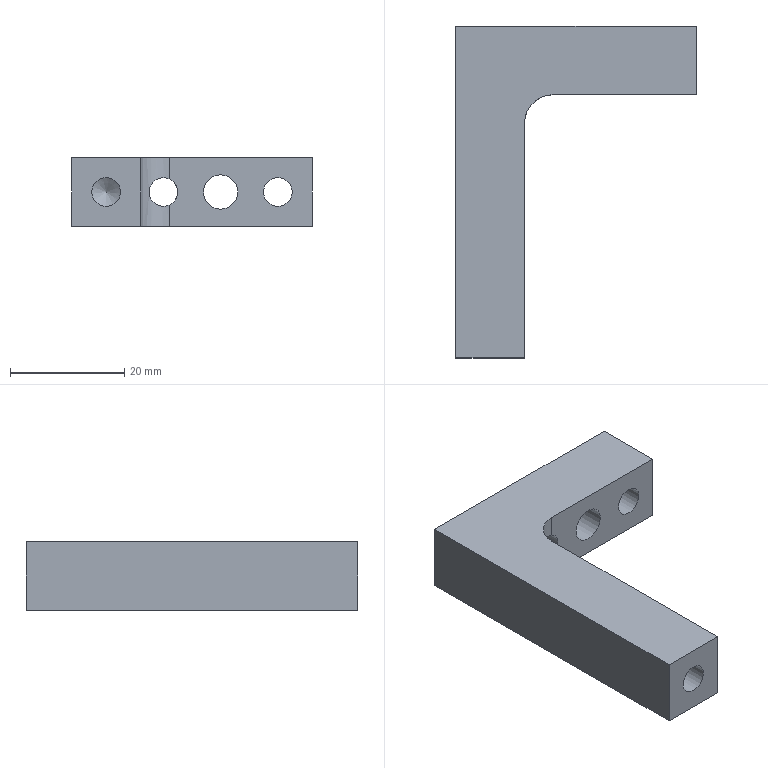Part | NX | features BREP 1 | 1 solid | 16 faces | box 42 x 58 x 12 mm | volume 11260 mm3 | plane 8 | cylinder 6 | cone 2 | commonest cylinder face diameters 5 x3 6 x2 10 x1
STEP:
#1=CARTESIAN_POINT('',(6.,0.,-3.5));
#2=VERTEX_POINT('',#1);
#3=CARTESIAN_POINT('',(6.,0.,-6.));
#4=DIRECTION('',(0.,1.,0.));
#5=DIRECTION('',(0.,0.,1.));
#6=AXIS2_PLACEMENT_3D('',#3,#4,#5);
#7=CIRCLE('',#6,2.5);
#8=EDGE_CURVE('',#2,#2,#7,.T.);
#9=ORIENTED_EDGE('',*,*,#8,.T.);
#10=EDGE_LOOP('',(#9));
#11=FACE_BOUND('',#10,.T.);
#12=CARTESIAN_POINT('',(0.,0.,0.));
#13=VERTEX_POINT('',#12);
#14=CARTESIAN_POINT('',(12.,0.,0.));
#15=VERTEX_POINT('',#14);
#16=CARTESIAN_POINT('',(12.,0.,0.));
#17=DIRECTION('',(1.,0.,0.));
#18=VECTOR('',#17,1000.);
#19=LINE('',#16,#18);
#20=EDGE_CURVE('',#13,#15,#19,.T.);
#21=ORIENTED_EDGE('',*,*,#20,.F.);
#22=CARTESIAN_POINT('',(0.,0.,-12.));
#23=VERTEX_POINT('',#22);
#24=CARTESIAN_POINT('',(0.,0.,-12.));
#25=DIRECTION('',(0.,0.,1.));
#26=VECTOR('',#25,1000.);
#27=LINE('',#24,#26);
#28=EDGE_CURVE('',#23,#13,#27,.T.);
#29=ORIENTED_EDGE('',*,*,#28,.F.);
#30=CARTESIAN_POINT('',(12.,0.,-12.));
#31=VERTEX_POINT('',#30);
#32=CARTESIAN_POINT('',(12.,0.,-12.));
#33=DIRECTION('',(1.,0.,0.));
#34=VECTOR('',#33,1000.);
#35=LINE('',#32,#34);
#36=EDGE_CURVE('',#23,#31,#35,.T.);
#37=ORIENTED_EDGE('',*,*,#36,.T.);
#38=CARTESIAN_POINT('',(12.,0.,-12.));
#39=DIRECTION('',(0.,0.,1.));
#40=VECTOR('',#39,1000.);
#41=LINE('',#38,#40);
#42=EDGE_CURVE('',#31,#15,#41,.T.);
#43=ORIENTED_EDGE('',*,*,#42,.T.);
#44=EDGE_LOOP('',(#21,#29,#37,#43));
#45=FACE_BOUND('',#44,.T.);
#46=CARTESIAN_POINT('',(12.,0.,-12.));
#47=DIRECTION('',(0.,1.,0.));
#48=DIRECTION('',(1.,0.,0.));
#49=AXIS2_PLACEMENT_3D('',#46,#47,#48);
#50=PLANE('',#49);
#51=ADVANCED_FACE('',(#11,#45),#50,.F.);
#52=CARTESIAN_POINT('',(12.,41.,0.));
#53=VERTEX_POINT('',#52);
#54=CARTESIAN_POINT('',(12.,46.,0.));
#55=DIRECTION('',(0.,1.,0.));
#56=VECTOR('',#55,1000.);
#57=LINE('',#54,#56);
#58=EDGE_CURVE('',#15,#53,#57,.T.);
#59=ORIENTED_EDGE('',*,*,#58,.F.);
#60=ORIENTED_EDGE('',*,*,#42,.F.);
#61=CARTESIAN_POINT('',(12.,41.,-12.));
#62=VERTEX_POINT('',#61);
#63=CARTESIAN_POINT('',(12.,46.,-12.));
#64=DIRECTION('',(0.,1.,0.));
#65=VECTOR('',#64,1000.);
#66=LINE('',#63,#65);
#67=EDGE_CURVE('',#31,#62,#66,.T.);
#68=ORIENTED_EDGE('',*,*,#67,.T.);
#69=CARTESIAN_POINT('',(12.,41.,-12.));
#70=DIRECTION('',(0.,0.,-1.));
#71=VECTOR('',#70,1000.);
#72=LINE('',#69,#71);
#73=EDGE_CURVE('',#53,#62,#72,.T.);
#74=ORIENTED_EDGE('',*,*,#73,.F.);
#75=EDGE_LOOP('',(#59,#60,#68,#74));
#76=FACE_BOUND('',#75,.T.);
#77=CARTESIAN_POINT('',(12.,46.,-12.));
#78=DIRECTION('',(-1.,0.,0.));
#79=DIRECTION('',(0.,1.,0.));
#80=AXIS2_PLACEMENT_3D('',#77,#78,#79);
#81=PLANE('',#80);
#82=ADVANCED_FACE('',(#76),#81,.F.);
#83=CARTESIAN_POINT('',(17.,46.,-12.));
#84=VERTEX_POINT('',#83);
#85=CARTESIAN_POINT('',(42.,46.,-12.));
#86=VERTEX_POINT('',#85);
#87=CARTESIAN_POINT('',(42.,46.,-12.));
#88=DIRECTION('',(1.,0.,0.));
#89=VECTOR('',#88,1000.);
#90=LINE('',#87,#89);
#91=EDGE_CURVE('',#84,#86,#90,.T.);
#92=ORIENTED_EDGE('',*,*,#91,.T.);
#93=CARTESIAN_POINT('',(42.,46.,0.));
#94=VERTEX_POINT('',#93);
#95=CARTESIAN_POINT('',(42.,46.,-12.));
#96=DIRECTION('',(0.,0.,1.));
#97=VECTOR('',#96,1000.);
#98=LINE('',#95,#97);
#99=EDGE_CURVE('',#86,#94,#98,.T.);
#100=ORIENTED_EDGE('',*,*,#99,.T.);
#101=CARTESIAN_POINT('',(17.,46.,0.));
#102=VERTEX_POINT('',#101);
#103=CARTESIAN_POINT('',(42.,46.,0.));
#104=DIRECTION('',(1.,0.,0.));
#105=VECTOR('',#104,1000.);
#106=LINE('',#103,#105);
#107=EDGE_CURVE('',#102,#94,#106,.T.);
#108=ORIENTED_EDGE('',*,*,#107,.F.);
#109=CARTESIAN_POINT('',(17.,46.,-3.709));
#110=VERTEX_POINT('',#109);
#111=CARTESIAN_POINT('',(17.,46.,0.));
#112=DIRECTION('',(0.,0.,1.));
#113=VECTOR('',#112,1000.);
#114=LINE('',#111,#113);
#115=EDGE_CURVE('',#110,#102,#114,.T.);
#116=ORIENTED_EDGE('',*,*,#115,.F.);
#117=CARTESIAN_POINT('',(17.,46.,-8.291));
#118=VERTEX_POINT('',#117);
#119=CARTESIAN_POINT('',(16.,46.,-6.));
#120=DIRECTION('',(0.,-1.,0.));
#121=DIRECTION('',(0.,0.,-1.));
#122=AXIS2_PLACEMENT_3D('',#119,#120,#121);
#123=CIRCLE('',#122,2.5);
#124=EDGE_CURVE('',#118,#110,#123,.T.);
#125=ORIENTED_EDGE('',*,*,#124,.F.);
#126=CARTESIAN_POINT('',(17.,46.,0.));
#127=DIRECTION('',(0.,0.,1.));
#128=VECTOR('',#127,1000.);
#129=LINE('',#126,#128);
#130=EDGE_CURVE('',#84,#118,#129,.T.);
#131=ORIENTED_EDGE('',*,*,#130,.F.);
#132=EDGE_LOOP('',(#92,#100,#108,#116,#125,#131));
#133=FACE_BOUND('',#132,.T.);
#134=CARTESIAN_POINT('',(36.,46.,-8.5));
#135=VERTEX_POINT('',#134);
#136=CARTESIAN_POINT('',(36.,46.,-6.));
#137=DIRECTION('',(0.,-1.,0.));
#138=DIRECTION('',(0.,0.,-1.));
#139=AXIS2_PLACEMENT_3D('',#136,#137,#138);
#140=CIRCLE('',#139,2.5);
#141=EDGE_CURVE('',#135,#135,#140,.T.);
#142=ORIENTED_EDGE('',*,*,#141,.F.);
#143=EDGE_LOOP('',(#142));
#144=FACE_BOUND('',#143,.T.);
#145=CARTESIAN_POINT('',(26.,46.,-9.));
#146=VERTEX_POINT('',#145);
#147=CARTESIAN_POINT('',(26.,46.,-6.));
#148=DIRECTION('',(0.,-1.,0.));
#149=DIRECTION('',(0.,0.,-1.));
#150=AXIS2_PLACEMENT_3D('',#147,#148,#149);
#151=CIRCLE('',#150,3.);
#152=EDGE_CURVE('',#146,#146,#151,.T.);
#153=ORIENTED_EDGE('',*,*,#152,.F.);
#154=EDGE_LOOP('',(#153));
#155=FACE_BOUND('',#154,.T.);
#156=CARTESIAN_POINT('',(42.,46.,-12.));
#157=DIRECTION('',(0.,1.,0.));
#158=DIRECTION('',(0.,0.,1.));
#159=AXIS2_PLACEMENT_3D('',#156,#157,#158);
#160=PLANE('',#159);
#161=ADVANCED_FACE('',(#133,#144,#155),#160,.F.);
#162=CARTESIAN_POINT('',(42.,58.,0.));
#163=VERTEX_POINT('',#162);
#164=CARTESIAN_POINT('',(42.,58.,0.));
#165=DIRECTION('',(0.,1.,0.));
#166=VECTOR('',#165,1000.);
#167=LINE('',#164,#166);
#168=EDGE_CURVE('',#94,#163,#167,.T.);
#169=ORIENTED_EDGE('',*,*,#168,.F.);
#170=ORIENTED_EDGE('',*,*,#99,.F.);
#171=CARTESIAN_POINT('',(42.,58.,-12.));
#172=VERTEX_POINT('',#171);
#173=CARTESIAN_POINT('',(42.,58.,-12.));
#174=DIRECTION('',(0.,1.,0.));
#175=VECTOR('',#174,1000.);
#176=LINE('',#173,#175);
#177=EDGE_CURVE('',#86,#172,#176,.T.);
#178=ORIENTED_EDGE('',*,*,#177,.T.);
#179=CARTESIAN_POINT('',(42.,58.,-12.));
#180=DIRECTION('',(0.,0.,1.));
#181=VECTOR('',#180,1000.);
#182=LINE('',#179,#181);
#183=EDGE_CURVE('',#172,#163,#182,.T.);
#184=ORIENTED_EDGE('',*,*,#183,.T.);
#185=EDGE_LOOP('',(#169,#170,#178,#184));
#186=FACE_BOUND('',#185,.T.);
#187=CARTESIAN_POINT('',(42.,58.,-12.));
#188=DIRECTION('',(-1.,0.,0.));
#189=DIRECTION('',(0.,1.,0.));
#190=AXIS2_PLACEMENT_3D('',#187,#188,#189);
#191=PLANE('',#190);
#192=ADVANCED_FACE('',(#186),#191,.F.);
#193=CARTESIAN_POINT('',(16.,58.,-8.5));
#194=VERTEX_POINT('',#193);
#195=CARTESIAN_POINT('',(16.,58.,-6.));
#196=DIRECTION('',(0.,-1.,0.));
#197=DIRECTION('',(0.,0.,-1.));
#198=AXIS2_PLACEMENT_3D('',#195,#196,#197);
#199=CIRCLE('',#198,2.5);
#200=EDGE_CURVE('',#194,#194,#199,.T.);
#201=ORIENTED_EDGE('',*,*,#200,.T.);
#202=EDGE_LOOP('',(#201));
#203=FACE_BOUND('',#202,.T.);
#204=CARTESIAN_POINT('',(36.,58.,-8.5));
#205=VERTEX_POINT('',#204);
#206=CARTESIAN_POINT('',(36.,58.,-6.));
#207=DIRECTION('',(0.,-1.,0.));
#208=DIRECTION('',(0.,0.,-1.));
#209=AXIS2_PLACEMENT_3D('',#206,#207,#208);
#210=CIRCLE('',#209,2.5);
#211=EDGE_CURVE('',#205,#205,#210,.T.);
#212=ORIENTED_EDGE('',*,*,#211,.T.);
#213=EDGE_LOOP('',(#212));
#214=FACE_BOUND('',#213,.T.);
#215=CARTESIAN_POINT('',(6.,58.,-9.));
#216=VERTEX_POINT('',#215);
#217=CARTESIAN_POINT('',(6.,58.,-6.));
#218=DIRECTION('',(0.,-1.,0.));
#219=DIRECTION('',(0.,0.,-1.));
#220=AXIS2_PLACEMENT_3D('',#217,#218,#219);
#221=CIRCLE('',#220,3.);
#222=EDGE_CURVE('',#216,#216,#221,.T.);
#223=ORIENTED_EDGE('',*,*,#222,.T.);
#224=EDGE_LOOP('',(#223));
#225=FACE_BOUND('',#224,.T.);
#226=CARTESIAN_POINT('',(26.,58.,-9.));
#227=VERTEX_POINT('',#226);
#228=CARTESIAN_POINT('',(26.,58.,-6.));
#229=DIRECTION('',(0.,-1.,0.));
#230=DIRECTION('',(0.,0.,-1.));
#231=AXIS2_PLACEMENT_3D('',#228,#229,#230);
#232=CIRCLE('',#231,3.);
#233=EDGE_CURVE('',#227,#227,#232,.T.);
#234=ORIENTED_EDGE('',*,*,#233,.T.);
#235=EDGE_LOOP('',(#234));
#236=FACE_BOUND('',#235,.T.);
#237=CARTESIAN_POINT('',(0.,58.,0.));
#238=VERTEX_POINT('',#237);
#239=CARTESIAN_POINT('',(0.,58.,0.));
#240=DIRECTION('',(-1.,0.,0.));
#241=VECTOR('',#240,1000.);
#242=LINE('',#239,#241);
#243=EDGE_CURVE('',#163,#238,#242,.T.);
#244=ORIENTED_EDGE('',*,*,#243,.F.);
#245=ORIENTED_EDGE('',*,*,#183,.F.);
#246=CARTESIAN_POINT('',(0.,58.,-12.));
#247=VERTEX_POINT('',#246);
#248=CARTESIAN_POINT('',(0.,58.,-12.));
#249=DIRECTION('',(-1.,0.,0.));
#250=VECTOR('',#249,1000.);
#251=LINE('',#248,#250);
#252=EDGE_CURVE('',#172,#247,#251,.T.);
#253=ORIENTED_EDGE('',*,*,#252,.T.);
#254=CARTESIAN_POINT('',(0.,58.,-12.));
#255=DIRECTION('',(0.,0.,1.));
#256=VECTOR('',#255,1000.);
#257=LINE('',#254,#256);
#258=EDGE_CURVE('',#247,#238,#257,.T.);
#259=ORIENTED_EDGE('',*,*,#258,.T.);
#260=EDGE_LOOP('',(#244,#245,#253,#259));
#261=FACE_BOUND('',#260,.T.);
#262=CARTESIAN_POINT('',(0.,58.,-12.));
#263=DIRECTION('',(0.,-1.,0.));
#264=DIRECTION('',(0.,0.,-1.));
#265=AXIS2_PLACEMENT_3D('',#262,#263,#264);
#266=PLANE('',#265);
#267=ADVANCED_FACE('',(#203,#214,#225,#236,#261),#266,.F.);
#268=CARTESIAN_POINT('',(0.,0.,0.));
#269=DIRECTION('',(0.,-1.,0.));
#270=VECTOR('',#269,1000.);
#271=LINE('',#268,#270);
#272=EDGE_CURVE('',#238,#13,#271,.T.);
#273=ORIENTED_EDGE('',*,*,#272,.F.);
#274=ORIENTED_EDGE('',*,*,#258,.F.);
#275=CARTESIAN_POINT('',(0.,0.,-12.));
#276=DIRECTION('',(0.,-1.,0.));
#277=VECTOR('',#276,1000.);
#278=LINE('',#275,#277);
#279=EDGE_CURVE('',#247,#23,#278,.T.);
#280=ORIENTED_EDGE('',*,*,#279,.T.);
#281=ORIENTED_EDGE('',*,*,#28,.T.);
#282=EDGE_LOOP('',(#273,#274,#280,#281));
#283=FACE_BOUND('',#282,.T.);
#284=CARTESIAN_POINT('',(0.,0.,-12.));
#285=DIRECTION('',(1.,0.,0.));
#286=DIRECTION('',(0.,0.,-1.));
#287=AXIS2_PLACEMENT_3D('',#284,#285,#286);
#288=PLANE('',#287);
#289=ADVANCED_FACE('',(#283),#288,.F.);
#290=ORIENTED_EDGE('',*,*,#36,.F.);
#291=ORIENTED_EDGE('',*,*,#279,.F.);
#292=ORIENTED_EDGE('',*,*,#252,.F.);
#293=ORIENTED_EDGE('',*,*,#177,.F.);
#294=ORIENTED_EDGE('',*,*,#91,.F.);
#295=CARTESIAN_POINT('',(17.,41.,-12.));
#296=DIRECTION('',(0.,0.,-1.));
#297=DIRECTION('',(-1.,0.,0.));
#298=AXIS2_PLACEMENT_3D('',#295,#296,#297);
#299=CIRCLE('',#298,5.);
#300=EDGE_CURVE('',#62,#84,#299,.T.);
#301=ORIENTED_EDGE('',*,*,#300,.F.);
#302=ORIENTED_EDGE('',*,*,#67,.F.);
#303=EDGE_LOOP('',(#290,#291,#292,#293,#294,#301,#302));
#304=FACE_BOUND('',#303,.T.);
#305=CARTESIAN_POINT('',(0.,0.,-12.));
#306=DIRECTION('',(0.,0.,1.));
#307=DIRECTION('',(1.,0.,0.));
#308=AXIS2_PLACEMENT_3D('',#305,#306,#307);
#309=PLANE('',#308);
#310=ADVANCED_FACE('',(#304),#309,.F.);
#311=ORIENTED_EDGE('',*,*,#20,.T.);
#312=ORIENTED_EDGE('',*,*,#58,.T.);
#313=CARTESIAN_POINT('',(17.,41.,0.));
#314=DIRECTION('',(0.,0.,1.));
#315=DIRECTION('',(-1.,0.,0.));
#316=AXIS2_PLACEMENT_3D('',#313,#314,#315);
#317=CIRCLE('',#316,5.);
#318=EDGE_CURVE('',#102,#53,#317,.T.);
#319=ORIENTED_EDGE('',*,*,#318,.F.);
#320=ORIENTED_EDGE('',*,*,#107,.T.);
#321=ORIENTED_EDGE('',*,*,#168,.T.);
#322=ORIENTED_EDGE('',*,*,#243,.T.);
#323=ORIENTED_EDGE('',*,*,#272,.T.);
#324=EDGE_LOOP('',(#311,#312,#319,#320,#321,#322,#323));
#325=FACE_BOUND('',#324,.T.);
#326=CARTESIAN_POINT('',(0.,0.,0.));
#327=DIRECTION('',(0.,0.,1.));
#328=DIRECTION('',(1.,0.,0.));
#329=AXIS2_PLACEMENT_3D('',#326,#327,#328);
#330=PLANE('',#329);
#331=ADVANCED_FACE('',(#325),#330,.T.);
#332=ORIENTED_EDGE('',*,*,#152,.T.);
#333=EDGE_LOOP('',(#332));
#334=FACE_BOUND('',#333,.T.);
#335=ORIENTED_EDGE('',*,*,#233,.F.);
#336=EDGE_LOOP('',(#335));
#337=FACE_BOUND('',#336,.T.);
#338=CARTESIAN_POINT('',(26.,58.,-6.));
#339=DIRECTION('',(0.,1.,0.));
#340=DIRECTION('',(0.,0.,1.));
#341=AXIS2_PLACEMENT_3D('',#338,#339,#340);
#342=CYLINDRICAL_SURFACE('',#341,3.);
#343=ADVANCED_FACE('',(#334,#337),#342,.F.);
#344=CARTESIAN_POINT('',(6.,44.197,-6.));
#345=VERTEX_POINT('',#344);
#346=VERTEX_LOOP('',#345);
#347=FACE_BOUND('',#346,.T.);
#348=CARTESIAN_POINT('',(6.,46.,-9.));
#349=VERTEX_POINT('',#348);
#350=CARTESIAN_POINT('',(6.,46.,-6.));
#351=DIRECTION('',(0.,-1.,0.));
#352=DIRECTION('',(0.,0.,-1.));
#353=AXIS2_PLACEMENT_3D('',#350,#351,#352);
#354=CIRCLE('',#353,3.);
#355=EDGE_CURVE('',#349,#349,#354,.T.);
#356=ORIENTED_EDGE('',*,*,#355,.F.);
#357=EDGE_LOOP('',(#356));
#358=FACE_BOUND('',#357,.T.);
#359=CARTESIAN_POINT('',(6.,46.,-6.));
#360=DIRECTION('',(0.,1.,0.));
#361=DIRECTION('',(0.,0.,1.));
#362=AXIS2_PLACEMENT_3D('',#359,#360,#361);
#363=CONICAL_SURFACE('',#362,3.,1.03);
#364=ADVANCED_FACE('',(#347,#358),#363,.F.);
#365=ORIENTED_EDGE('',*,*,#355,.T.);
#366=EDGE_LOOP('',(#365));
#367=FACE_BOUND('',#366,.T.);
#368=ORIENTED_EDGE('',*,*,#222,.F.);
#369=EDGE_LOOP('',(#368));
#370=FACE_BOUND('',#369,.T.);
#371=CARTESIAN_POINT('',(6.,58.,-6.));
#372=DIRECTION('',(0.,1.,0.));
#373=DIRECTION('',(0.,0.,1.));
#374=AXIS2_PLACEMENT_3D('',#371,#372,#373);
#375=CYLINDRICAL_SURFACE('',#374,3.);
#376=ADVANCED_FACE('',(#367,#370),#375,.F.);
#377=ORIENTED_EDGE('',*,*,#211,.F.);
#378=EDGE_LOOP('',(#377));
#379=FACE_BOUND('',#378,.T.);
#380=ORIENTED_EDGE('',*,*,#141,.T.);
#381=EDGE_LOOP('',(#380));
#382=FACE_BOUND('',#381,.T.);
#383=CARTESIAN_POINT('',(36.,58.,-6.));
#384=DIRECTION('',(0.,1.,0.));
#385=DIRECTION('',(0.,0.,1.));
#386=AXIS2_PLACEMENT_3D('',#383,#384,#385);
#387=CYLINDRICAL_SURFACE('',#386,2.5);
#388=ADVANCED_FACE('',(#379,#382),#387,.F.);
#389=ORIENTED_EDGE('',*,*,#200,.F.);
#390=EDGE_LOOP('',(#389));
#391=FACE_BOUND('',#390,.T.);
#392=ORIENTED_EDGE('',*,*,#124,.T.);
#393=CARTESIAN_POINT('',(17.,46.,-8.291));
#394=CARTESIAN_POINT('',(16.197,46.,-8.642));
#395=CARTESIAN_POINT('',(14.806,45.612,-8.438));
#396=CARTESIAN_POINT('',(13.74,44.814,-7.281));
#397=CARTESIAN_POINT('',(13.38,44.449,-6.002));
#398=CARTESIAN_POINT('',(13.739,44.813,-4.721));
#399=CARTESIAN_POINT('',(14.808,45.613,-3.561));
#400=CARTESIAN_POINT('',(16.196,46.,-3.358));
#401=CARTESIAN_POINT('',(17.,46.,-3.709));
#402=B_SPLINE_CURVE_WITH_KNOTS('',3,(#393,#394,#395,#396,#397,#398,#399,#400,#401),.UNSPECIFIED.,.F.,.F.,(4,1,1,1,1,1,4),(0.,0.002589,0.003884,0.005179,0.006474,0.007768,0.01036),.UNSPECIFIED.);
#403=EDGE_CURVE('',#118,#110,#402,.T.);
#404=ORIENTED_EDGE('',*,*,#403,.F.);
#405=EDGE_LOOP('',(#392,#404));
#406=FACE_BOUND('',#405,.T.);
#407=CARTESIAN_POINT('',(16.,58.,-6.));
#408=DIRECTION('',(0.,1.,0.));
#409=DIRECTION('',(0.,0.,1.));
#410=AXIS2_PLACEMENT_3D('',#407,#408,#409);
#411=CYLINDRICAL_SURFACE('',#410,2.5);
#412=ADVANCED_FACE('',(#391,#406),#411,.F.);
#413=ORIENTED_EDGE('',*,*,#300,.T.);
#414=ORIENTED_EDGE('',*,*,#130,.T.);
#415=ORIENTED_EDGE('',*,*,#403,.T.);
#416=ORIENTED_EDGE('',*,*,#115,.T.);
#417=ORIENTED_EDGE('',*,*,#318,.T.);
#418=ORIENTED_EDGE('',*,*,#73,.T.);
#419=EDGE_LOOP('',(#413,#414,#415,#416,#417,#418));
#420=FACE_BOUND('',#419,.T.);
#421=CARTESIAN_POINT('',(17.,41.,-12.));
#422=DIRECTION('',(0.,0.,-1.));
#423=DIRECTION('',(-1.,0.,0.));
#424=AXIS2_PLACEMENT_3D('',#421,#422,#423);
#425=CYLINDRICAL_SURFACE('',#424,5.);
#426=ADVANCED_FACE('',(#420),#425,.F.);
#427=CARTESIAN_POINT('',(6.,16.502,-6.));
#428=VERTEX_POINT('',#427);
#429=VERTEX_LOOP('',#428);
#430=FACE_BOUND('',#429,.T.);
#431=CARTESIAN_POINT('',(6.,15.,-3.5));
#432=VERTEX_POINT('',#431);
#433=CARTESIAN_POINT('',(6.,15.,-6.));
#434=DIRECTION('',(0.,1.,0.));
#435=DIRECTION('',(0.,0.,1.));
#436=AXIS2_PLACEMENT_3D('',#433,#434,#435);
#437=CIRCLE('',#436,2.5);
#438=EDGE_CURVE('',#432,#432,#437,.T.);
#439=ORIENTED_EDGE('',*,*,#438,.F.);
#440=EDGE_LOOP('',(#439));
#441=FACE_BOUND('',#440,.T.);
#442=CARTESIAN_POINT('',(6.,15.,-6.));
#443=DIRECTION('',(0.,-1.,0.));
#444=DIRECTION('',(0.,0.,-1.));
#445=AXIS2_PLACEMENT_3D('',#442,#443,#444);
#446=CONICAL_SURFACE('',#445,2.5,1.03);
#447=ADVANCED_FACE('',(#430,#441),#446,.F.);
#448=ORIENTED_EDGE('',*,*,#438,.T.);
#449=EDGE_LOOP('',(#448));
#450=FACE_BOUND('',#449,.T.);
#451=ORIENTED_EDGE('',*,*,#8,.F.);
#452=EDGE_LOOP('',(#451));
#453=FACE_BOUND('',#452,.T.);
#454=CARTESIAN_POINT('',(6.,0.,-6.));
#455=DIRECTION('',(0.,-1.,0.));
#456=DIRECTION('',(0.,0.,-1.));
#457=AXIS2_PLACEMENT_3D('',#454,#455,#456);
#458=CYLINDRICAL_SURFACE('',#457,2.5);
#459=ADVANCED_FACE('',(#450,#453),#458,.F.);
#460=CLOSED_SHELL('',(#51,#82,#161,#192,#267,#289,#310,#331,#343,#364,#376,#388,#412,#426,#447,#459));
#461=MANIFOLD_SOLID_BREP('',#460);
#462=(LENGTH_UNIT()NAMED_UNIT(*)SI_UNIT(.MILLI.,.METRE.));
#463=UNCERTAINTY_MEASURE_WITH_UNIT(LENGTH_MEASURE(0.0508),#462,'','');
#464=(NAMED_UNIT(*)PLANE_ANGLE_UNIT()SI_UNIT($,.RADIAN.));
#465=(NAMED_UNIT(*)SI_UNIT($,.STERADIAN.)SOLID_ANGLE_UNIT());
#466=(GEOMETRIC_REPRESENTATION_CONTEXT(3)GLOBAL_UNCERTAINTY_ASSIGNED_CONTEXT((#463))GLOBAL_UNIT_ASSIGNED_CONTEXT((#462,#464,#465))REPRESENTATION_CONTEXT('',''));
#467=ADVANCED_BREP_SHAPE_REPRESENTATION('',(#461),#466);